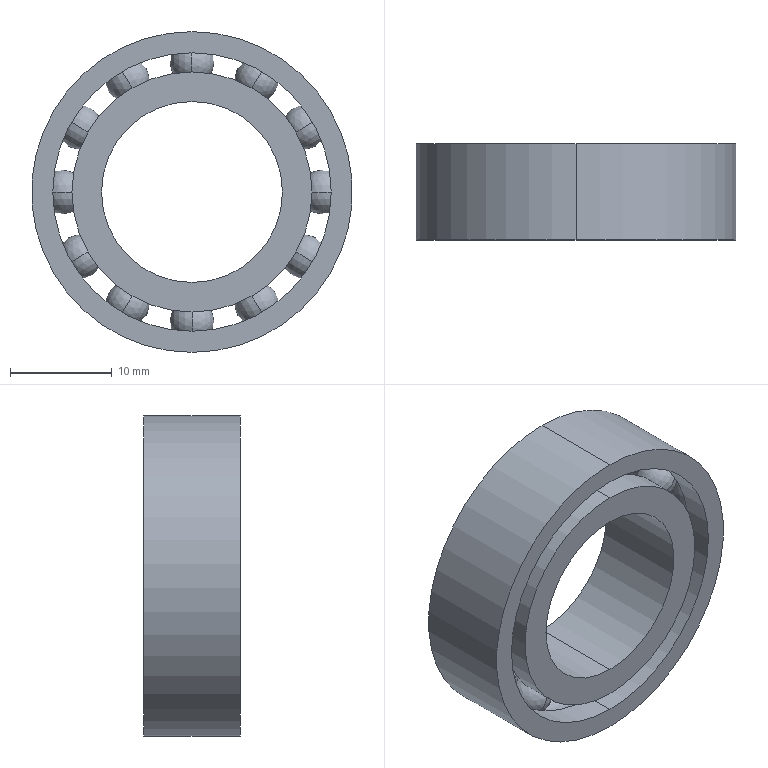Part | SolidWorks | features SavedExtBody 14 | 14 solids | 46 faces | box 31.502 x 9.43 x 31.502 mm | volume 3555 mm3 | sphere 24 | cylinder 12 | torus 6 | plane 4 | commonest cylinder face diameters 23.576 x4 27.342 x4 17.774 x2 31.502 x2
STEP:
#1=CARTESIAN_POINT('',(-11.024,-216.87,71.365));
#2=VERTEX_POINT('',#1);
#3=CARTESIAN_POINT('',(-11.024,-212.601,71.365));
#4=VERTEX_POINT('',#3);
#5=CARTESIAN_POINT('',(-11.024,-214.736,71.365));
#6=DIRECTION('',(0.5,0.,0.866));
#7=DIRECTION('',(0.866,0.,-0.5));
#8=AXIS2_PLACEMENT_3D('',#5,#6,#7);
#9=CIRCLE('',#8,2.135);
#10=EDGE_CURVE('',#2,#4,#9,.T.);
#11=ORIENTED_EDGE('',*,*,#10,.F.);
#12=CARTESIAN_POINT('',(-11.024,-214.736,71.365));
#13=DIRECTION('',(-0.5,0.,-0.866));
#14=DIRECTION('',(-0.866,0.,0.5));
#15=AXIS2_PLACEMENT_3D('',#12,#13,#14);
#16=CIRCLE('',#15,2.135);
#17=EDGE_CURVE('',#2,#4,#16,.T.);
#18=ORIENTED_EDGE('',*,*,#17,.T.);
#19=EDGE_LOOP('',(#11,#18));
#20=FACE_OUTER_BOUND('',#19,.T.);
#21=CARTESIAN_POINT('',(-11.024,-214.736,71.365));
#22=DIRECTION('',(-0.5,0.,-0.866));
#23=DIRECTION('',(0.866,0.,-0.5));
#24=AXIS2_PLACEMENT_3D('',#21,#22,#23);
#25=SPHERICAL_SURFACE('',#24,2.135);
#26=ADVANCED_FACE('',(#20),#25,.T.);
#27=ORIENTED_EDGE('',*,*,#17,.F.);
#28=ORIENTED_EDGE('',*,*,#10,.T.);
#29=EDGE_LOOP('',(#27,#28));
#30=FACE_OUTER_BOUND('',#29,.T.);
#31=CARTESIAN_POINT('',(-11.024,-214.736,71.365));
#32=DIRECTION('',(-0.5,0.,-0.866));
#33=DIRECTION('',(0.866,0.,-0.5));
#34=AXIS2_PLACEMENT_3D('',#31,#32,#33);
#35=SPHERICAL_SURFACE('',#34,2.135);
#36=ADVANCED_FACE('',(#30),#35,.T.);
#37=CLOSED_SHELL('',(#26,#36));
#38=MANIFOLD_SOLID_BREP('',#37);
#39=CARTESIAN_POINT('',(-6.365,-216.87,76.024));
#40=VERTEX_POINT('',#39);
#41=CARTESIAN_POINT('',(-6.365,-212.601,76.024));
#42=VERTEX_POINT('',#41);
#43=CARTESIAN_POINT('',(-6.365,-214.736,76.024));
#44=DIRECTION('',(0.866,0.,0.5));
#45=DIRECTION('',(0.5,0.,-0.866));
#46=AXIS2_PLACEMENT_3D('',#43,#44,#45);
#47=CIRCLE('',#46,2.135);
#48=EDGE_CURVE('',#40,#42,#47,.T.);
#49=ORIENTED_EDGE('',*,*,#48,.F.);
#50=CARTESIAN_POINT('',(-6.365,-214.736,76.024));
#51=DIRECTION('',(-0.866,0.,-0.5));
#52=DIRECTION('',(-0.5,0.,0.866));
#53=AXIS2_PLACEMENT_3D('',#50,#51,#52);
#54=CIRCLE('',#53,2.135);
#55=EDGE_CURVE('',#40,#42,#54,.T.);
#56=ORIENTED_EDGE('',*,*,#55,.T.);
#57=EDGE_LOOP('',(#49,#56));
#58=FACE_OUTER_BOUND('',#57,.T.);
#59=CARTESIAN_POINT('',(-6.365,-214.736,76.024));
#60=DIRECTION('',(-0.866,0.,-0.5));
#61=DIRECTION('',(0.5,0.,-0.866));
#62=AXIS2_PLACEMENT_3D('',#59,#60,#61);
#63=SPHERICAL_SURFACE('',#62,2.135);
#64=ADVANCED_FACE('',(#58),#63,.T.);
#65=ORIENTED_EDGE('',*,*,#55,.F.);
#66=ORIENTED_EDGE('',*,*,#48,.T.);
#67=EDGE_LOOP('',(#65,#66));
#68=FACE_OUTER_BOUND('',#67,.T.);
#69=CARTESIAN_POINT('',(-6.365,-214.736,76.024));
#70=DIRECTION('',(-0.866,0.,-0.5));
#71=DIRECTION('',(0.5,0.,-0.866));
#72=AXIS2_PLACEMENT_3D('',#69,#70,#71);
#73=SPHERICAL_SURFACE('',#72,2.135);
#74=ADVANCED_FACE('',(#68),#73,.T.);
#75=CLOSED_SHELL('',(#64,#74));
#76=MANIFOLD_SOLID_BREP('',#75);
#77=CARTESIAN_POINT('',(0.,-216.87,77.729));
#78=VERTEX_POINT('',#77);
#79=CARTESIAN_POINT('',(0.,-212.601,77.729));
#80=VERTEX_POINT('',#79);
#81=CARTESIAN_POINT('',(0.,-214.736,77.729));
#82=DIRECTION('',(1.,0.,0.));
#83=DIRECTION('',(0.,0.,-1.));
#84=AXIS2_PLACEMENT_3D('',#81,#82,#83);
#85=CIRCLE('',#84,2.135);
#86=EDGE_CURVE('',#78,#80,#85,.T.);
#87=ORIENTED_EDGE('',*,*,#86,.F.);
#88=CARTESIAN_POINT('',(0.,-214.736,77.729));
#89=DIRECTION('',(-1.,0.,0.));
#90=DIRECTION('',(0.,0.,1.));
#91=AXIS2_PLACEMENT_3D('',#88,#89,#90);
#92=CIRCLE('',#91,2.135);
#93=EDGE_CURVE('',#78,#80,#92,.T.);
#94=ORIENTED_EDGE('',*,*,#93,.T.);
#95=EDGE_LOOP('',(#87,#94));
#96=FACE_OUTER_BOUND('',#95,.T.);
#97=CARTESIAN_POINT('',(0.,-214.736,77.729));
#98=DIRECTION('',(-1.,0.,0.));
#99=DIRECTION('',(0.,0.,-1.));
#100=AXIS2_PLACEMENT_3D('',#97,#98,#99);
#101=SPHERICAL_SURFACE('',#100,2.135);
#102=ADVANCED_FACE('',(#96),#101,.T.);
#103=ORIENTED_EDGE('',*,*,#93,.F.);
#104=ORIENTED_EDGE('',*,*,#86,.T.);
#105=EDGE_LOOP('',(#103,#104));
#106=FACE_OUTER_BOUND('',#105,.T.);
#107=CARTESIAN_POINT('',(0.,-214.736,77.729));
#108=DIRECTION('',(-1.,0.,0.));
#109=DIRECTION('',(0.,0.,-1.));
#110=AXIS2_PLACEMENT_3D('',#107,#108,#109);
#111=SPHERICAL_SURFACE('',#110,2.135);
#112=ADVANCED_FACE('',(#106),#111,.T.);
#113=CLOSED_SHELL('',(#102,#112));
#114=MANIFOLD_SOLID_BREP('',#113);
#115=CARTESIAN_POINT('',(6.365,-216.87,76.024));
#116=VERTEX_POINT('',#115);
#117=CARTESIAN_POINT('',(6.365,-212.601,76.024));
#118=VERTEX_POINT('',#117);
#119=CARTESIAN_POINT('',(6.365,-214.736,76.024));
#120=DIRECTION('',(0.866,0.,-0.5));
#121=DIRECTION('',(-0.5,0.,-0.866));
#122=AXIS2_PLACEMENT_3D('',#119,#120,#121);
#123=CIRCLE('',#122,2.135);
#124=EDGE_CURVE('',#116,#118,#123,.T.);
#125=ORIENTED_EDGE('',*,*,#124,.F.);
#126=CARTESIAN_POINT('',(6.365,-214.736,76.024));
#127=DIRECTION('',(-0.866,0.,0.5));
#128=DIRECTION('',(0.5,0.,0.866));
#129=AXIS2_PLACEMENT_3D('',#126,#127,#128);
#130=CIRCLE('',#129,2.135);
#131=EDGE_CURVE('',#116,#118,#130,.T.);
#132=ORIENTED_EDGE('',*,*,#131,.T.);
#133=EDGE_LOOP('',(#125,#132));
#134=FACE_OUTER_BOUND('',#133,.T.);
#135=CARTESIAN_POINT('',(6.365,-214.736,76.024));
#136=DIRECTION('',(-0.866,0.,0.5));
#137=DIRECTION('',(-0.5,0.,-0.866));
#138=AXIS2_PLACEMENT_3D('',#135,#136,#137);
#139=SPHERICAL_SURFACE('',#138,2.135);
#140=ADVANCED_FACE('',(#134),#139,.T.);
#141=ORIENTED_EDGE('',*,*,#131,.F.);
#142=ORIENTED_EDGE('',*,*,#124,.T.);
#143=EDGE_LOOP('',(#141,#142));
#144=FACE_OUTER_BOUND('',#143,.T.);
#145=CARTESIAN_POINT('',(6.365,-214.736,76.024));
#146=DIRECTION('',(-0.866,0.,0.5));
#147=DIRECTION('',(-0.5,0.,-0.866));
#148=AXIS2_PLACEMENT_3D('',#145,#146,#147);
#149=SPHERICAL_SURFACE('',#148,2.135);
#150=ADVANCED_FACE('',(#144),#149,.T.);
#151=CLOSED_SHELL('',(#140,#150));
#152=MANIFOLD_SOLID_BREP('',#151);
#153=CARTESIAN_POINT('',(11.024,-216.87,71.365));
#154=VERTEX_POINT('',#153);
#155=CARTESIAN_POINT('',(11.024,-212.601,71.365));
#156=VERTEX_POINT('',#155);
#157=CARTESIAN_POINT('',(11.024,-214.736,71.365));
#158=DIRECTION('',(0.5,0.,-0.866));
#159=DIRECTION('',(-0.866,0.,-0.5));
#160=AXIS2_PLACEMENT_3D('',#157,#158,#159);
#161=CIRCLE('',#160,2.135);
#162=EDGE_CURVE('',#154,#156,#161,.T.);
#163=ORIENTED_EDGE('',*,*,#162,.F.);
#164=CARTESIAN_POINT('',(11.024,-214.736,71.365));
#165=DIRECTION('',(-0.5,0.,0.866));
#166=DIRECTION('',(0.866,0.,0.5));
#167=AXIS2_PLACEMENT_3D('',#164,#165,#166);
#168=CIRCLE('',#167,2.135);
#169=EDGE_CURVE('',#154,#156,#168,.T.);
#170=ORIENTED_EDGE('',*,*,#169,.T.);
#171=EDGE_LOOP('',(#163,#170));
#172=FACE_OUTER_BOUND('',#171,.T.);
#173=CARTESIAN_POINT('',(11.024,-214.736,71.365));
#174=DIRECTION('',(-0.5,0.,0.866));
#175=DIRECTION('',(-0.866,0.,-0.5));
#176=AXIS2_PLACEMENT_3D('',#173,#174,#175);
#177=SPHERICAL_SURFACE('',#176,2.135);
#178=ADVANCED_FACE('',(#172),#177,.T.);
#179=ORIENTED_EDGE('',*,*,#169,.F.);
#180=ORIENTED_EDGE('',*,*,#162,.T.);
#181=EDGE_LOOP('',(#179,#180));
#182=FACE_OUTER_BOUND('',#181,.T.);
#183=CARTESIAN_POINT('',(11.024,-214.736,71.365));
#184=DIRECTION('',(-0.5,0.,0.866));
#185=DIRECTION('',(-0.866,0.,-0.5));
#186=AXIS2_PLACEMENT_3D('',#183,#184,#185);
#187=SPHERICAL_SURFACE('',#186,2.135);
#188=ADVANCED_FACE('',(#182),#187,.T.);
#189=CLOSED_SHELL('',(#178,#188));
#190=MANIFOLD_SOLID_BREP('',#189);
#191=CARTESIAN_POINT('',(12.729,-216.87,65.));
#192=VERTEX_POINT('',#191);
#193=CARTESIAN_POINT('',(12.729,-212.601,65.));
#194=VERTEX_POINT('',#193);
#195=CARTESIAN_POINT('',(12.729,-214.736,65.));
#196=DIRECTION('',(0.,0.,-1.));
#197=DIRECTION('',(-1.,0.,0.));
#198=AXIS2_PLACEMENT_3D('',#195,#196,#197);
#199=CIRCLE('',#198,2.135);
#200=EDGE_CURVE('',#192,#194,#199,.T.);
#201=ORIENTED_EDGE('',*,*,#200,.F.);
#202=CARTESIAN_POINT('',(12.729,-214.736,65.));
#203=DIRECTION('',(0.,0.,1.));
#204=DIRECTION('',(1.,0.,0.));
#205=AXIS2_PLACEMENT_3D('',#202,#203,#204);
#206=CIRCLE('',#205,2.135);
#207=EDGE_CURVE('',#192,#194,#206,.T.);
#208=ORIENTED_EDGE('',*,*,#207,.T.);
#209=EDGE_LOOP('',(#201,#208));
#210=FACE_OUTER_BOUND('',#209,.T.);
#211=CARTESIAN_POINT('',(12.729,-214.736,65.));
#212=DIRECTION('',(0.,0.,1.));
#213=DIRECTION('',(-1.,0.,0.));
#214=AXIS2_PLACEMENT_3D('',#211,#212,#213);
#215=SPHERICAL_SURFACE('',#214,2.135);
#216=ADVANCED_FACE('',(#210),#215,.T.);
#217=ORIENTED_EDGE('',*,*,#207,.F.);
#218=ORIENTED_EDGE('',*,*,#200,.T.);
#219=EDGE_LOOP('',(#217,#218));
#220=FACE_OUTER_BOUND('',#219,.T.);
#221=CARTESIAN_POINT('',(12.729,-214.736,65.));
#222=DIRECTION('',(0.,0.,1.));
#223=DIRECTION('',(-1.,0.,0.));
#224=AXIS2_PLACEMENT_3D('',#221,#222,#223);
#225=SPHERICAL_SURFACE('',#224,2.135);
#226=ADVANCED_FACE('',(#220),#225,.T.);
#227=CLOSED_SHELL('',(#216,#226));
#228=MANIFOLD_SOLID_BREP('',#227);
#229=CARTESIAN_POINT('',(6.365,-216.87,53.976));
#230=VERTEX_POINT('',#229);
#231=CARTESIAN_POINT('',(6.365,-212.601,53.976));
#232=VERTEX_POINT('',#231);
#233=CARTESIAN_POINT('',(6.365,-214.736,53.976));
#234=DIRECTION('',(-0.866,0.,-0.5));
#235=DIRECTION('',(-0.5,0.,0.866));
#236=AXIS2_PLACEMENT_3D('',#233,#234,#235);
#237=CIRCLE('',#236,2.135);
#238=EDGE_CURVE('',#230,#232,#237,.T.);
#239=ORIENTED_EDGE('',*,*,#238,.F.);
#240=CARTESIAN_POINT('',(6.365,-214.736,53.976));
#241=DIRECTION('',(0.866,0.,0.5));
#242=DIRECTION('',(0.5,0.,-0.866));
#243=AXIS2_PLACEMENT_3D('',#240,#241,#242);
#244=CIRCLE('',#243,2.135);
#245=EDGE_CURVE('',#230,#232,#244,.T.);
#246=ORIENTED_EDGE('',*,*,#245,.T.);
#247=EDGE_LOOP('',(#239,#246));
#248=FACE_OUTER_BOUND('',#247,.T.);
#249=CARTESIAN_POINT('',(6.365,-214.736,53.976));
#250=DIRECTION('',(0.866,0.,0.5));
#251=DIRECTION('',(-0.5,0.,0.866));
#252=AXIS2_PLACEMENT_3D('',#249,#250,#251);
#253=SPHERICAL_SURFACE('',#252,2.135);
#254=ADVANCED_FACE('',(#248),#253,.T.);
#255=ORIENTED_EDGE('',*,*,#245,.F.);
#256=ORIENTED_EDGE('',*,*,#238,.T.);
#257=EDGE_LOOP('',(#255,#256));
#258=FACE_OUTER_BOUND('',#257,.T.);
#259=CARTESIAN_POINT('',(6.365,-214.736,53.976));
#260=DIRECTION('',(0.866,0.,0.5));
#261=DIRECTION('',(-0.5,0.,0.866));
#262=AXIS2_PLACEMENT_3D('',#259,#260,#261);
#263=SPHERICAL_SURFACE('',#262,2.135);
#264=ADVANCED_FACE('',(#258),#263,.T.);
#265=CLOSED_SHELL('',(#254,#264));
#266=MANIFOLD_SOLID_BREP('',#265);
#267=CARTESIAN_POINT('',(0.,-216.87,52.271));
#268=VERTEX_POINT('',#267);
#269=CARTESIAN_POINT('',(0.,-212.601,52.271));
#270=VERTEX_POINT('',#269);
#271=CARTESIAN_POINT('',(0.,-214.736,52.271));
#272=DIRECTION('',(-1.,0.,0.));
#273=DIRECTION('',(0.,0.,1.));
#274=AXIS2_PLACEMENT_3D('',#271,#272,#273);
#275=CIRCLE('',#274,2.135);
#276=EDGE_CURVE('',#268,#270,#275,.T.);
#277=ORIENTED_EDGE('',*,*,#276,.F.);
#278=CARTESIAN_POINT('',(0.,-214.736,52.271));
#279=DIRECTION('',(1.,0.,0.));
#280=DIRECTION('',(0.,0.,-1.));
#281=AXIS2_PLACEMENT_3D('',#278,#279,#280);
#282=CIRCLE('',#281,2.135);
#283=EDGE_CURVE('',#268,#270,#282,.T.);
#284=ORIENTED_EDGE('',*,*,#283,.T.);
#285=EDGE_LOOP('',(#277,#284));
#286=FACE_OUTER_BOUND('',#285,.T.);
#287=CARTESIAN_POINT('',(0.,-214.736,52.271));
#288=DIRECTION('',(1.,0.,0.));
#289=DIRECTION('',(0.,0.,1.));
#290=AXIS2_PLACEMENT_3D('',#287,#288,#289);
#291=SPHERICAL_SURFACE('',#290,2.135);
#292=ADVANCED_FACE('',(#286),#291,.T.);
#293=ORIENTED_EDGE('',*,*,#283,.F.);
#294=ORIENTED_EDGE('',*,*,#276,.T.);
#295=EDGE_LOOP('',(#293,#294));
#296=FACE_OUTER_BOUND('',#295,.T.);
#297=CARTESIAN_POINT('',(0.,-214.736,52.271));
#298=DIRECTION('',(1.,0.,0.));
#299=DIRECTION('',(0.,0.,1.));
#300=AXIS2_PLACEMENT_3D('',#297,#298,#299);
#301=SPHERICAL_SURFACE('',#300,2.135);
#302=ADVANCED_FACE('',(#296),#301,.T.);
#303=CLOSED_SHELL('',(#292,#302));
#304=MANIFOLD_SOLID_BREP('',#303);
#305=CARTESIAN_POINT('',(-6.365,-216.87,53.976));
#306=VERTEX_POINT('',#305);
#307=CARTESIAN_POINT('',(-6.365,-212.601,53.976));
#308=VERTEX_POINT('',#307);
#309=CARTESIAN_POINT('',(-6.365,-214.736,53.976));
#310=DIRECTION('',(-0.866,0.,0.5));
#311=DIRECTION('',(0.5,0.,0.866));
#312=AXIS2_PLACEMENT_3D('',#309,#310,#311);
#313=CIRCLE('',#312,2.135);
#314=EDGE_CURVE('',#306,#308,#313,.T.);
#315=ORIENTED_EDGE('',*,*,#314,.F.);
#316=CARTESIAN_POINT('',(-6.365,-214.736,53.976));
#317=DIRECTION('',(0.866,0.,-0.5));
#318=DIRECTION('',(-0.5,0.,-0.866));
#319=AXIS2_PLACEMENT_3D('',#316,#317,#318);
#320=CIRCLE('',#319,2.135);
#321=EDGE_CURVE('',#306,#308,#320,.T.);
#322=ORIENTED_EDGE('',*,*,#321,.T.);
#323=EDGE_LOOP('',(#315,#322));
#324=FACE_OUTER_BOUND('',#323,.T.);
#325=CARTESIAN_POINT('',(-6.365,-214.736,53.976));
#326=DIRECTION('',(0.866,0.,-0.5));
#327=DIRECTION('',(0.5,0.,0.866));
#328=AXIS2_PLACEMENT_3D('',#325,#326,#327);
#329=SPHERICAL_SURFACE('',#328,2.135);
#330=ADVANCED_FACE('',(#324),#329,.T.);
#331=ORIENTED_EDGE('',*,*,#321,.F.);
#332=ORIENTED_EDGE('',*,*,#314,.T.);
#333=EDGE_LOOP('',(#331,#332));
#334=FACE_OUTER_BOUND('',#333,.T.);
#335=CARTESIAN_POINT('',(-6.365,-214.736,53.976));
#336=DIRECTION('',(0.866,0.,-0.5));
#337=DIRECTION('',(0.5,0.,0.866));
#338=AXIS2_PLACEMENT_3D('',#335,#336,#337);
#339=SPHERICAL_SURFACE('',#338,2.135);
#340=ADVANCED_FACE('',(#334),#339,.T.);
#341=CLOSED_SHELL('',(#330,#340));
#342=MANIFOLD_SOLID_BREP('',#341);
#343=CARTESIAN_POINT('',(-11.024,-216.87,58.635));
#344=VERTEX_POINT('',#343);
#345=CARTESIAN_POINT('',(-11.024,-212.601,58.635));
#346=VERTEX_POINT('',#345);
#347=CARTESIAN_POINT('',(-11.024,-214.736,58.635));
#348=DIRECTION('',(-0.5,0.,0.866));
#349=DIRECTION('',(0.866,0.,0.5));
#350=AXIS2_PLACEMENT_3D('',#347,#348,#349);
#351=CIRCLE('',#350,2.135);
#352=EDGE_CURVE('',#344,#346,#351,.T.);
#353=ORIENTED_EDGE('',*,*,#352,.F.);
#354=CARTESIAN_POINT('',(-11.024,-214.736,58.635));
#355=DIRECTION('',(0.5,0.,-0.866));
#356=DIRECTION('',(-0.866,0.,-0.5));
#357=AXIS2_PLACEMENT_3D('',#354,#355,#356);
#358=CIRCLE('',#357,2.135);
#359=EDGE_CURVE('',#344,#346,#358,.T.);
#360=ORIENTED_EDGE('',*,*,#359,.T.);
#361=EDGE_LOOP('',(#353,#360));
#362=FACE_OUTER_BOUND('',#361,.T.);
#363=CARTESIAN_POINT('',(-11.024,-214.736,58.635));
#364=DIRECTION('',(0.5,0.,-0.866));
#365=DIRECTION('',(0.866,0.,0.5));
#366=AXIS2_PLACEMENT_3D('',#363,#364,#365);
#367=SPHERICAL_SURFACE('',#366,2.135);
#368=ADVANCED_FACE('',(#362),#367,.T.);
#369=ORIENTED_EDGE('',*,*,#359,.F.);
#370=ORIENTED_EDGE('',*,*,#352,.T.);
#371=EDGE_LOOP('',(#369,#370));
#372=FACE_OUTER_BOUND('',#371,.T.);
#373=CARTESIAN_POINT('',(-11.024,-214.736,58.635));
#374=DIRECTION('',(0.5,0.,-0.866));
#375=DIRECTION('',(0.866,0.,0.5));
#376=AXIS2_PLACEMENT_3D('',#373,#374,#375);
#377=SPHERICAL_SURFACE('',#376,2.135);
#378=ADVANCED_FACE('',(#372),#377,.T.);
#379=CLOSED_SHELL('',(#368,#378));
#380=MANIFOLD_SOLID_BREP('',#379);
#381=CARTESIAN_POINT('',(-12.729,-216.87,65.));
#382=VERTEX_POINT('',#381);
#383=CARTESIAN_POINT('',(-12.729,-212.601,65.));
#384=VERTEX_POINT('',#383);
#385=CARTESIAN_POINT('',(-12.729,-214.736,65.));
#386=DIRECTION('',(0.,0.,1.));
#387=DIRECTION('',(1.,0.,0.));
#388=AXIS2_PLACEMENT_3D('',#385,#386,#387);
#389=CIRCLE('',#388,2.135);
#390=EDGE_CURVE('',#382,#384,#389,.T.);
#391=ORIENTED_EDGE('',*,*,#390,.F.);
#392=CARTESIAN_POINT('',(-12.729,-214.736,65.));
#393=DIRECTION('',(0.,0.,-1.));
#394=DIRECTION('',(-1.,0.,0.));
#395=AXIS2_PLACEMENT_3D('',#392,#393,#394);
#396=CIRCLE('',#395,2.135);
#397=EDGE_CURVE('',#382,#384,#396,.T.);
#398=ORIENTED_EDGE('',*,*,#397,.T.);
#399=EDGE_LOOP('',(#391,#398));
#400=FACE_OUTER_BOUND('',#399,.T.);
#401=CARTESIAN_POINT('',(-12.729,-214.736,65.));
#402=DIRECTION('',(0.,0.,-1.));
#403=DIRECTION('',(1.,0.,0.));
#404=AXIS2_PLACEMENT_3D('',#401,#402,#403);
#405=SPHERICAL_SURFACE('',#404,2.135);
#406=ADVANCED_FACE('',(#400),#405,.T.);
#407=ORIENTED_EDGE('',*,*,#397,.F.);
#408=ORIENTED_EDGE('',*,*,#390,.T.);
#409=EDGE_LOOP('',(#407,#408));
#410=FACE_OUTER_BOUND('',#409,.T.);
#411=CARTESIAN_POINT('',(-12.729,-214.736,65.));
#412=DIRECTION('',(0.,0.,-1.));
#413=DIRECTION('',(1.,0.,0.));
#414=AXIS2_PLACEMENT_3D('',#411,#412,#413);
#415=SPHERICAL_SURFACE('',#414,2.135);
#416=ADVANCED_FACE('',(#410),#415,.T.);
#417=CLOSED_SHELL('',(#406,#416));
#418=MANIFOLD_SOLID_BREP('',#417);
#419=CARTESIAN_POINT('',(0.,-216.652,53.212));
#420=VERTEX_POINT('',#419);
#421=CARTESIAN_POINT('',(0.,-214.736,54.405));
#422=VERTEX_POINT('',#421);
#423=CARTESIAN_POINT('',(0.,-214.736,52.271));
#424=DIRECTION('',(-1.,0.,0.));
#425=DIRECTION('',(0.,0.,1.));
#426=AXIS2_PLACEMENT_3D('',#423,#424,#425);
#427=CIRCLE('',#426,2.135);
#428=EDGE_CURVE('',#420,#422,#427,.T.);
#429=ORIENTED_EDGE('',*,*,#428,.T.);
#430=CARTESIAN_POINT('',(0.,-214.736,75.595));
#431=VERTEX_POINT('',#430);
#432=CARTESIAN_POINT('',(0.,-214.736,65.));
#433=DIRECTION('',(0.,-1.,0.));
#434=DIRECTION('',(0.,0.,-1.));
#435=AXIS2_PLACEMENT_3D('',#432,#433,#434);
#436=CIRCLE('',#435,10.595);
#437=EDGE_CURVE('',#422,#431,#436,.T.);
#438=ORIENTED_EDGE('',*,*,#437,.T.);
#439=CARTESIAN_POINT('',(0.,-216.652,76.788));
#440=VERTEX_POINT('',#439);
#441=CARTESIAN_POINT('',(0.,-214.736,77.729));
#442=DIRECTION('',(1.,0.,0.));
#443=DIRECTION('',(0.,0.,-1.));
#444=AXIS2_PLACEMENT_3D('',#441,#442,#443);
#445=CIRCLE('',#444,2.135);
#446=EDGE_CURVE('',#440,#431,#445,.T.);
#447=ORIENTED_EDGE('',*,*,#446,.F.);
#448=CARTESIAN_POINT('',(0.,-216.652,65.));
#449=DIRECTION('',(0.,-1.,0.));
#450=DIRECTION('',(0.,0.,-1.));
#451=AXIS2_PLACEMENT_3D('',#448,#449,#450);
#452=CIRCLE('',#451,11.788);
#453=EDGE_CURVE('',#420,#440,#452,.T.);
#454=ORIENTED_EDGE('',*,*,#453,.F.);
#455=EDGE_LOOP('',(#429,#438,#447,#454));
#456=FACE_OUTER_BOUND('',#455,.T.);
#457=CARTESIAN_POINT('',(0.,-214.736,65.));
#458=DIRECTION('',(0.,-1.,0.));
#459=DIRECTION('',(0.,0.,-1.));
#460=AXIS2_PLACEMENT_3D('',#457,#458,#459);
#461=TOROIDAL_SURFACE('',#460,12.729,2.135);
#462=ADVANCED_FACE('',(#456),#461,.F.);
#463=ORIENTED_EDGE('',*,*,#446,.T.);
#464=CARTESIAN_POINT('',(0.,-214.736,65.));
#465=DIRECTION('',(0.,-1.,0.));
#466=DIRECTION('',(0.,0.,-1.));
#467=AXIS2_PLACEMENT_3D('',#464,#465,#466);
#468=CIRCLE('',#467,10.595);
#469=EDGE_CURVE('',#431,#422,#468,.T.);
#470=ORIENTED_EDGE('',*,*,#469,.T.);
#471=ORIENTED_EDGE('',*,*,#428,.F.);
#472=CARTESIAN_POINT('',(0.,-216.652,65.));
#473=DIRECTION('',(0.,-1.,0.));
#474=DIRECTION('',(0.,0.,-1.));
#475=AXIS2_PLACEMENT_3D('',#472,#473,#474);
#476=CIRCLE('',#475,11.788);
#477=EDGE_CURVE('',#440,#420,#476,.T.);
#478=ORIENTED_EDGE('',*,*,#477,.F.);
#479=EDGE_LOOP('',(#463,#470,#471,#478));
#480=FACE_OUTER_BOUND('',#479,.T.);
#481=CARTESIAN_POINT('',(0.,-214.736,65.));
#482=DIRECTION('',(0.,-1.,0.));
#483=DIRECTION('',(0.,0.,-1.));
#484=AXIS2_PLACEMENT_3D('',#481,#482,#483);
#485=TOROIDAL_SURFACE('',#484,12.729,2.135);
#486=ADVANCED_FACE('',(#480),#485,.F.);
#487=CARTESIAN_POINT('',(0.,-210.021,73.887));
#488=VERTEX_POINT('',#487);
#489=CARTESIAN_POINT('',(0.,-210.021,56.113));
#490=VERTEX_POINT('',#489);
#491=CARTESIAN_POINT('',(0.,-210.021,65.));
#492=DIRECTION('',(0.,-1.,0.));
#493=DIRECTION('',(0.,0.,-1.));
#494=AXIS2_PLACEMENT_3D('',#491,#492,#493);
#495=CIRCLE('',#494,8.887);
#496=EDGE_CURVE('',#488,#490,#495,.T.);
#497=ORIENTED_EDGE('',*,*,#496,.F.);
#498=CARTESIAN_POINT('',(0.,-219.451,73.887));
#499=VERTEX_POINT('',#498);
#500=CARTESIAN_POINT('',(0.,-253.035,73.887));
#501=DIRECTION('',(0.,-1.,0.));
#502=VECTOR('',#501,1000.);
#503=LINE('',#500,#502);
#504=EDGE_CURVE('',#488,#499,#503,.T.);
#505=ORIENTED_EDGE('',*,*,#504,.T.);
#506=CARTESIAN_POINT('',(0.,-219.451,56.113));
#507=VERTEX_POINT('',#506);
#508=CARTESIAN_POINT('',(0.,-219.451,65.));
#509=DIRECTION('',(0.,-1.,0.));
#510=DIRECTION('',(0.,0.,-1.));
#511=AXIS2_PLACEMENT_3D('',#508,#509,#510);
#512=CIRCLE('',#511,8.887);
#513=EDGE_CURVE('',#499,#507,#512,.T.);
#514=ORIENTED_EDGE('',*,*,#513,.T.);
#515=CARTESIAN_POINT('',(0.,-253.035,56.113));
#516=DIRECTION('',(0.,-1.,0.));
#517=VECTOR('',#516,1000.);
#518=LINE('',#515,#517);
#519=EDGE_CURVE('',#490,#507,#518,.T.);
#520=ORIENTED_EDGE('',*,*,#519,.F.);
#521=EDGE_LOOP('',(#497,#505,#514,#520));
#522=FACE_OUTER_BOUND('',#521,.T.);
#523=CARTESIAN_POINT('',(0.,-253.035,65.));
#524=DIRECTION('',(0.,-1.,0.));
#525=DIRECTION('',(0.,0.,-1.));
#526=AXIS2_PLACEMENT_3D('',#523,#524,#525);
#527=CYLINDRICAL_SURFACE('',#526,8.887);
#528=ADVANCED_FACE('',(#522),#527,.F.);
#529=ORIENTED_EDGE('',*,*,#453,.T.);
#530=CARTESIAN_POINT('',(0.,-219.451,76.788));
#531=VERTEX_POINT('',#530);
#532=CARTESIAN_POINT('',(0.,-253.035,76.788));
#533=DIRECTION('',(0.,-1.,0.));
#534=VECTOR('',#533,1000.);
#535=LINE('',#532,#534);
#536=EDGE_CURVE('',#440,#531,#535,.T.);
#537=ORIENTED_EDGE('',*,*,#536,.T.);
#538=CARTESIAN_POINT('',(0.,-219.451,53.212));
#539=VERTEX_POINT('',#538);
#540=CARTESIAN_POINT('',(0.,-219.451,65.));
#541=DIRECTION('',(0.,-1.,0.));
#542=DIRECTION('',(0.,0.,-1.));
#543=AXIS2_PLACEMENT_3D('',#540,#541,#542);
#544=CIRCLE('',#543,11.788);
#545=EDGE_CURVE('',#539,#531,#544,.T.);
#546=ORIENTED_EDGE('',*,*,#545,.F.);
#547=CARTESIAN_POINT('',(0.,-253.035,53.212));
#548=DIRECTION('',(0.,-1.,0.));
#549=VECTOR('',#548,1000.);
#550=LINE('',#547,#549);
#551=EDGE_CURVE('',#420,#539,#550,.T.);
#552=ORIENTED_EDGE('',*,*,#551,.F.);
#553=EDGE_LOOP('',(#529,#537,#546,#552));
#554=FACE_OUTER_BOUND('',#553,.T.);
#555=CARTESIAN_POINT('',(0.,-253.035,65.));
#556=DIRECTION('',(0.,-1.,0.));
#557=DIRECTION('',(0.,0.,-1.));
#558=AXIS2_PLACEMENT_3D('',#555,#556,#557);
#559=CYLINDRICAL_SURFACE('',#558,11.788);
#560=ADVANCED_FACE('',(#554),#559,.T.);
#561=ORIENTED_EDGE('',*,*,#469,.F.);
#562=CARTESIAN_POINT('',(0.,-212.82,76.788));
#563=VERTEX_POINT('',#562);
#564=CARTESIAN_POINT('',(0.,-214.736,77.729));
#565=DIRECTION('',(1.,0.,0.));
#566=DIRECTION('',(0.,0.,-1.));
#567=AXIS2_PLACEMENT_3D('',#564,#565,#566);
#568=CIRCLE('',#567,2.135);
#569=EDGE_CURVE('',#431,#563,#568,.T.);
#570=ORIENTED_EDGE('',*,*,#569,.T.);
#571=CARTESIAN_POINT('',(0.,-212.82,53.212));
#572=VERTEX_POINT('',#571);
#573=CARTESIAN_POINT('',(0.,-212.82,65.));
#574=DIRECTION('',(0.,-1.,0.));
#575=DIRECTION('',(0.,0.,-1.));
#576=AXIS2_PLACEMENT_3D('',#573,#574,#575);
#577=CIRCLE('',#576,11.788);
#578=EDGE_CURVE('',#563,#572,#577,.T.);
#579=ORIENTED_EDGE('',*,*,#578,.T.);
#580=CARTESIAN_POINT('',(0.,-214.736,52.271));
#581=DIRECTION('',(-1.,0.,0.));
#582=DIRECTION('',(0.,0.,1.));
#583=AXIS2_PLACEMENT_3D('',#580,#581,#582);
#584=CIRCLE('',#583,2.135);
#585=EDGE_CURVE('',#422,#572,#584,.T.);
#586=ORIENTED_EDGE('',*,*,#585,.F.);
#587=EDGE_LOOP('',(#561,#570,#579,#586));
#588=FACE_OUTER_BOUND('',#587,.T.);
#589=CARTESIAN_POINT('',(0.,-214.736,65.));
#590=DIRECTION('',(0.,-1.,0.));
#591=DIRECTION('',(0.,0.,-1.));
#592=AXIS2_PLACEMENT_3D('',#589,#590,#591);
#593=TOROIDAL_SURFACE('',#592,12.729,2.135);
#594=ADVANCED_FACE('',(#588),#593,.F.);
#595=CARTESIAN_POINT('',(0.,-210.021,53.212));
#596=VERTEX_POINT('',#595);
#597=CARTESIAN_POINT('',(0.,-210.021,76.788));
#598=VERTEX_POINT('',#597);
#599=CARTESIAN_POINT('',(0.,-210.021,65.));
#600=DIRECTION('',(0.,-1.,0.));
#601=DIRECTION('',(0.,0.,-1.));
#602=AXIS2_PLACEMENT_3D('',#599,#600,#601);
#603=CIRCLE('',#602,11.788);
#604=EDGE_CURVE('',#596,#598,#603,.T.);
#605=ORIENTED_EDGE('',*,*,#604,.T.);
#606=CARTESIAN_POINT('',(0.,-253.035,76.788));
#607=DIRECTION('',(0.,-1.,0.));
#608=VECTOR('',#607,1000.);
#609=LINE('',#606,#608);
#610=EDGE_CURVE('',#598,#563,#609,.T.);
#611=ORIENTED_EDGE('',*,*,#610,.T.);
#612=CARTESIAN_POINT('',(0.,-212.82,65.));
#613=DIRECTION('',(0.,-1.,0.));
#614=DIRECTION('',(0.,0.,-1.));
#615=AXIS2_PLACEMENT_3D('',#612,#613,#614);
#616=CIRCLE('',#615,11.788);
#617=EDGE_CURVE('',#572,#563,#616,.T.);
#618=ORIENTED_EDGE('',*,*,#617,.F.);
#619=CARTESIAN_POINT('',(0.,-253.035,53.212));
#620=DIRECTION('',(0.,-1.,0.));
#621=VECTOR('',#620,1000.);
#622=LINE('',#619,#621);
#623=EDGE_CURVE('',#596,#572,#622,.T.);
#624=ORIENTED_EDGE('',*,*,#623,.F.);
#625=EDGE_LOOP('',(#605,#611,#618,#624));
#626=FACE_OUTER_BOUND('',#625,.T.);
#627=CARTESIAN_POINT('',(0.,-253.035,65.));
#628=DIRECTION('',(0.,-1.,0.));
#629=DIRECTION('',(0.,0.,-1.));
#630=AXIS2_PLACEMENT_3D('',#627,#628,#629);
#631=CYLINDRICAL_SURFACE('',#630,11.788);
#632=ADVANCED_FACE('',(#626),#631,.T.);
#633=ORIENTED_EDGE('',*,*,#604,.F.);
#634=CARTESIAN_POINT('',(0.,-210.021,65.));
#635=DIRECTION('',(0.,-1.,0.));
#636=DIRECTION('',(0.,0.,-1.));
#637=AXIS2_PLACEMENT_3D('',#634,#635,#636);
#638=CIRCLE('',#637,11.788);
#639=EDGE_CURVE('',#598,#596,#638,.T.);
#640=ORIENTED_EDGE('',*,*,#639,.F.);
#641=EDGE_LOOP('',(#633,#640));
#642=FACE_OUTER_BOUND('',#641,.T.);
#643=CARTESIAN_POINT('',(0.,-210.021,65.));
#644=DIRECTION('',(0.,-1.,0.));
#645=DIRECTION('',(0.,0.,-1.));
#646=AXIS2_PLACEMENT_3D('',#643,#644,#645);
#647=CIRCLE('',#646,8.887);
#648=EDGE_CURVE('',#490,#488,#647,.T.);
#649=ORIENTED_EDGE('',*,*,#648,.T.);
#650=ORIENTED_EDGE('',*,*,#496,.T.);
#651=EDGE_LOOP('',(#649,#650));
#652=FACE_BOUND('',#651,.T.);
#653=CARTESIAN_POINT('',(-11.788,-210.021,65.));
#654=DIRECTION('',(0.,-1.,0.));
#655=DIRECTION('',(0.,0.,-1.));
#656=AXIS2_PLACEMENT_3D('',#653,#654,#655);
#657=PLANE('',#656);
#658=ADVANCED_FACE('',(#642,#652),#657,.F.);
#659=ORIENTED_EDGE('',*,*,#610,.F.);
#660=ORIENTED_EDGE('',*,*,#639,.T.);
#661=ORIENTED_EDGE('',*,*,#623,.T.);
#662=ORIENTED_EDGE('',*,*,#578,.F.);
#663=EDGE_LOOP('',(#659,#660,#661,#662));
#664=FACE_OUTER_BOUND('',#663,.T.);
#665=CARTESIAN_POINT('',(0.,-253.035,65.));
#666=DIRECTION('',(0.,-1.,0.));
#667=DIRECTION('',(0.,0.,-1.));
#668=AXIS2_PLACEMENT_3D('',#665,#666,#667);
#669=CYLINDRICAL_SURFACE('',#668,11.788);
#670=ADVANCED_FACE('',(#664),#669,.T.);
#671=ORIENTED_EDGE('',*,*,#437,.F.);
#672=ORIENTED_EDGE('',*,*,#585,.T.);
#673=ORIENTED_EDGE('',*,*,#617,.T.);
#674=ORIENTED_EDGE('',*,*,#569,.F.);
#675=EDGE_LOOP('',(#671,#672,#673,#674));
#676=FACE_OUTER_BOUND('',#675,.T.);
#677=CARTESIAN_POINT('',(0.,-214.736,65.));
#678=DIRECTION('',(0.,-1.,0.));
#679=DIRECTION('',(0.,0.,-1.));
#680=AXIS2_PLACEMENT_3D('',#677,#678,#679);
#681=TOROIDAL_SURFACE('',#680,12.729,2.135);
#682=ADVANCED_FACE('',(#676),#681,.F.);
#683=ORIENTED_EDGE('',*,*,#536,.F.);
#684=ORIENTED_EDGE('',*,*,#477,.T.);
#685=ORIENTED_EDGE('',*,*,#551,.T.);
#686=CARTESIAN_POINT('',(0.,-219.451,65.));
#687=DIRECTION('',(0.,-1.,0.));
#688=DIRECTION('',(0.,0.,-1.));
#689=AXIS2_PLACEMENT_3D('',#686,#687,#688);
#690=CIRCLE('',#689,11.788);
#691=EDGE_CURVE('',#531,#539,#690,.T.);
#692=ORIENTED_EDGE('',*,*,#691,.F.);
#693=EDGE_LOOP('',(#683,#684,#685,#692));
#694=FACE_OUTER_BOUND('',#693,.T.);
#695=CARTESIAN_POINT('',(0.,-253.035,65.));
#696=DIRECTION('',(0.,-1.,0.));
#697=DIRECTION('',(0.,0.,-1.));
#698=AXIS2_PLACEMENT_3D('',#695,#696,#697);
#699=CYLINDRICAL_SURFACE('',#698,11.788);
#700=ADVANCED_FACE('',(#694),#699,.T.);
#701=CARTESIAN_POINT('',(0.,-219.451,65.));
#702=DIRECTION('',(0.,-1.,0.));
#703=DIRECTION('',(0.,0.,-1.));
#704=AXIS2_PLACEMENT_3D('',#701,#702,#703);
#705=CIRCLE('',#704,8.887);
#706=EDGE_CURVE('',#507,#499,#705,.T.);
#707=ORIENTED_EDGE('',*,*,#706,.F.);
#708=ORIENTED_EDGE('',*,*,#513,.F.);
#709=EDGE_LOOP('',(#707,#708));
#710=FACE_BOUND('',#709,.T.);
#711=ORIENTED_EDGE('',*,*,#545,.T.);
#712=ORIENTED_EDGE('',*,*,#691,.T.);
#713=EDGE_LOOP('',(#711,#712));
#714=FACE_OUTER_BOUND('',#713,.T.);
#715=CARTESIAN_POINT('',(-11.788,-219.451,65.));
#716=DIRECTION('',(0.,1.,0.));
#717=DIRECTION('',(0.,0.,1.));
#718=AXIS2_PLACEMENT_3D('',#715,#716,#717);
#719=PLANE('',#718);
#720=ADVANCED_FACE('',(#710,#714),#719,.F.);
#721=ORIENTED_EDGE('',*,*,#504,.F.);
#722=ORIENTED_EDGE('',*,*,#648,.F.);
#723=ORIENTED_EDGE('',*,*,#519,.T.);
#724=ORIENTED_EDGE('',*,*,#706,.T.);
#725=EDGE_LOOP('',(#721,#722,#723,#724));
#726=FACE_OUTER_BOUND('',#725,.T.);
#727=CARTESIAN_POINT('',(0.,-253.035,65.));
#728=DIRECTION('',(0.,-1.,0.));
#729=DIRECTION('',(0.,0.,-1.));
#730=AXIS2_PLACEMENT_3D('',#727,#728,#729);
#731=CYLINDRICAL_SURFACE('',#730,8.887);
#732=ADVANCED_FACE('',(#726),#731,.F.);
#733=CLOSED_SHELL('',(#462,#486,#528,#560,#594,#632,#658,#670,#682,#700,#720,#732));
#734=MANIFOLD_SOLID_BREP('',#733);
#735=CARTESIAN_POINT('',(0.,-210.021,78.671));
#736=VERTEX_POINT('',#735);
#737=CARTESIAN_POINT('',(0.,-210.021,51.329));
#738=VERTEX_POINT('',#737);
#739=CARTESIAN_POINT('',(0.,-210.021,65.));
#740=DIRECTION('',(0.,-1.,0.));
#741=DIRECTION('',(0.,0.,-1.));
#742=AXIS2_PLACEMENT_3D('',#739,#740,#741);
#743=CIRCLE('',#742,13.671);
#744=EDGE_CURVE('',#736,#738,#743,.T.);
#745=ORIENTED_EDGE('',*,*,#744,.F.);
#746=CARTESIAN_POINT('',(0.,-212.82,78.671));
#747=VERTEX_POINT('',#746);
#748=CARTESIAN_POINT('',(0.,-253.035,78.671));
#749=DIRECTION('',(0.,-1.,0.));
#750=VECTOR('',#749,1000.);
#751=LINE('',#748,#750);
#752=EDGE_CURVE('',#736,#747,#751,.T.);
#753=ORIENTED_EDGE('',*,*,#752,.T.);
#754=CARTESIAN_POINT('',(0.,-212.82,51.329));
#755=VERTEX_POINT('',#754);
#756=CARTESIAN_POINT('',(0.,-212.82,65.));
#757=DIRECTION('',(0.,-1.,0.));
#758=DIRECTION('',(0.,0.,-1.));
#759=AXIS2_PLACEMENT_3D('',#756,#757,#758);
#760=CIRCLE('',#759,13.671);
#761=EDGE_CURVE('',#747,#755,#760,.T.);
#762=ORIENTED_EDGE('',*,*,#761,.T.);
#763=CARTESIAN_POINT('',(0.,-253.035,51.329));
#764=DIRECTION('',(0.,-1.,0.));
#765=VECTOR('',#764,1000.);
#766=LINE('',#763,#765);
#767=EDGE_CURVE('',#738,#755,#766,.T.);
#768=ORIENTED_EDGE('',*,*,#767,.F.);
#769=EDGE_LOOP('',(#745,#753,#762,#768));
#770=FACE_OUTER_BOUND('',#769,.T.);
#771=CARTESIAN_POINT('',(0.,-253.035,65.));
#772=DIRECTION('',(0.,-1.,0.));
#773=DIRECTION('',(0.,0.,-1.));
#774=AXIS2_PLACEMENT_3D('',#771,#772,#773);
#775=CYLINDRICAL_SURFACE('',#774,13.671);
#776=ADVANCED_FACE('',(#770),#775,.F.);
#777=ORIENTED_EDGE('',*,*,#761,.F.);
#778=CARTESIAN_POINT('',(0.,-216.652,78.671));
#779=VERTEX_POINT('',#778);
#780=CARTESIAN_POINT('',(0.,-214.736,77.729));
#781=DIRECTION('',(1.,0.,0.));
#782=DIRECTION('',(0.,0.,-1.));
#783=AXIS2_PLACEMENT_3D('',#780,#781,#782);
#784=CIRCLE('',#783,2.135);
#785=EDGE_CURVE('',#747,#779,#784,.T.);
#786=ORIENTED_EDGE('',*,*,#785,.T.);
#787=CARTESIAN_POINT('',(0.,-216.652,51.329));
#788=VERTEX_POINT('',#787);
#789=CARTESIAN_POINT('',(0.,-216.652,65.));
#790=DIRECTION('',(0.,-1.,0.));
#791=DIRECTION('',(0.,0.,-1.));
#792=AXIS2_PLACEMENT_3D('',#789,#790,#791);
#793=CIRCLE('',#792,13.671);
#794=EDGE_CURVE('',#779,#788,#793,.T.);
#795=ORIENTED_EDGE('',*,*,#794,.T.);
#796=CARTESIAN_POINT('',(0.,-214.736,52.271));
#797=DIRECTION('',(-1.,0.,0.));
#798=DIRECTION('',(0.,0.,1.));
#799=AXIS2_PLACEMENT_3D('',#796,#797,#798);
#800=CIRCLE('',#799,2.135);
#801=EDGE_CURVE('',#755,#788,#800,.T.);
#802=ORIENTED_EDGE('',*,*,#801,.F.);
#803=EDGE_LOOP('',(#777,#786,#795,#802));
#804=FACE_OUTER_BOUND('',#803,.T.);
#805=CARTESIAN_POINT('',(0.,-214.736,65.));
#806=DIRECTION('',(0.,-1.,0.));
#807=DIRECTION('',(0.,0.,-1.));
#808=AXIS2_PLACEMENT_3D('',#805,#806,#807);
#809=TOROIDAL_SURFACE('',#808,12.729,2.135);
#810=ADVANCED_FACE('',(#804),#809,.F.);
#811=ORIENTED_EDGE('',*,*,#794,.F.);
#812=CARTESIAN_POINT('',(0.,-219.451,78.671));
#813=VERTEX_POINT('',#812);
#814=CARTESIAN_POINT('',(0.,-253.035,78.671));
#815=DIRECTION('',(0.,-1.,0.));
#816=VECTOR('',#815,1000.);
#817=LINE('',#814,#816);
#818=EDGE_CURVE('',#779,#813,#817,.T.);
#819=ORIENTED_EDGE('',*,*,#818,.T.);
#820=CARTESIAN_POINT('',(0.,-219.451,51.329));
#821=VERTEX_POINT('',#820);
#822=CARTESIAN_POINT('',(0.,-219.451,65.));
#823=DIRECTION('',(0.,-1.,0.));
#824=DIRECTION('',(0.,0.,-1.));
#825=AXIS2_PLACEMENT_3D('',#822,#823,#824);
#826=CIRCLE('',#825,13.671);
#827=EDGE_CURVE('',#813,#821,#826,.T.);
#828=ORIENTED_EDGE('',*,*,#827,.T.);
#829=CARTESIAN_POINT('',(0.,-253.035,51.329));
#830=DIRECTION('',(0.,-1.,0.));
#831=VECTOR('',#830,1000.);
#832=LINE('',#829,#831);
#833=EDGE_CURVE('',#788,#821,#832,.T.);
#834=ORIENTED_EDGE('',*,*,#833,.F.);
#835=EDGE_LOOP('',(#811,#819,#828,#834));
#836=FACE_OUTER_BOUND('',#835,.T.);
#837=CARTESIAN_POINT('',(0.,-253.035,65.));
#838=DIRECTION('',(0.,-1.,0.));
#839=DIRECTION('',(0.,0.,-1.));
#840=AXIS2_PLACEMENT_3D('',#837,#838,#839);
#841=CYLINDRICAL_SURFACE('',#840,13.671);
#842=ADVANCED_FACE('',(#836),#841,.F.);
#843=CARTESIAN_POINT('',(0.,-210.021,49.249));
#844=VERTEX_POINT('',#843);
#845=CARTESIAN_POINT('',(0.,-210.021,80.751));
#846=VERTEX_POINT('',#845);
#847=CARTESIAN_POINT('',(0.,-210.021,65.));
#848=DIRECTION('',(0.,-1.,0.));
#849=DIRECTION('',(0.,0.,-1.));
#850=AXIS2_PLACEMENT_3D('',#847,#848,#849);
#851=CIRCLE('',#850,15.751);
#852=EDGE_CURVE('',#844,#846,#851,.T.);
#853=ORIENTED_EDGE('',*,*,#852,.T.);
#854=CARTESIAN_POINT('',(0.,-219.451,80.751));
#855=VERTEX_POINT('',#854);
#856=CARTESIAN_POINT('',(0.,-253.035,80.751));
#857=DIRECTION('',(0.,-1.,0.));
#858=VECTOR('',#857,1000.);
#859=LINE('',#856,#858);
#860=EDGE_CURVE('',#846,#855,#859,.T.);
#861=ORIENTED_EDGE('',*,*,#860,.T.);
#862=CARTESIAN_POINT('',(0.,-219.451,49.249));
#863=VERTEX_POINT('',#862);
#864=CARTESIAN_POINT('',(0.,-219.451,65.));
#865=DIRECTION('',(0.,-1.,0.));
#866=DIRECTION('',(0.,0.,-1.));
#867=AXIS2_PLACEMENT_3D('',#864,#865,#866);
#868=CIRCLE('',#867,15.751);
#869=EDGE_CURVE('',#863,#855,#868,.T.);
#870=ORIENTED_EDGE('',*,*,#869,.F.);
#871=CARTESIAN_POINT('',(0.,-253.035,49.249));
#872=DIRECTION('',(0.,-1.,0.));
#873=VECTOR('',#872,1000.);
#874=LINE('',#871,#873);
#875=EDGE_CURVE('',#844,#863,#874,.T.);
#876=ORIENTED_EDGE('',*,*,#875,.F.);
#877=EDGE_LOOP('',(#853,#861,#870,#876));
#878=FACE_OUTER_BOUND('',#877,.T.);
#879=CARTESIAN_POINT('',(0.,-253.035,65.));
#880=DIRECTION('',(0.,-1.,0.));
#881=DIRECTION('',(0.,0.,-1.));
#882=AXIS2_PLACEMENT_3D('',#879,#880,#881);
#883=CYLINDRICAL_SURFACE('',#882,15.751);
#884=ADVANCED_FACE('',(#878),#883,.T.);
#885=ORIENTED_EDGE('',*,*,#860,.F.);
#886=CARTESIAN_POINT('',(0.,-210.021,65.));
#887=DIRECTION('',(0.,-1.,0.));
#888=DIRECTION('',(0.,0.,-1.));
#889=AXIS2_PLACEMENT_3D('',#886,#887,#888);
#890=CIRCLE('',#889,15.751);
#891=EDGE_CURVE('',#846,#844,#890,.T.);
#892=ORIENTED_EDGE('',*,*,#891,.T.);
#893=ORIENTED_EDGE('',*,*,#875,.T.);
#894=CARTESIAN_POINT('',(0.,-219.451,65.));
#895=DIRECTION('',(0.,-1.,0.));
#896=DIRECTION('',(0.,0.,-1.));
#897=AXIS2_PLACEMENT_3D('',#894,#895,#896);
#898=CIRCLE('',#897,15.751);
#899=EDGE_CURVE('',#855,#863,#898,.T.);
#900=ORIENTED_EDGE('',*,*,#899,.F.);
#901=EDGE_LOOP('',(#885,#892,#893,#900));
#902=FACE_OUTER_BOUND('',#901,.T.);
#903=CARTESIAN_POINT('',(0.,-253.035,65.));
#904=DIRECTION('',(0.,-1.,0.));
#905=DIRECTION('',(0.,0.,-1.));
#906=AXIS2_PLACEMENT_3D('',#903,#904,#905);
#907=CYLINDRICAL_SURFACE('',#906,15.751);
#908=ADVANCED_FACE('',(#902),#907,.T.);
#909=CARTESIAN_POINT('',(0.,-219.451,65.));
#910=DIRECTION('',(0.,-1.,0.));
#911=DIRECTION('',(0.,0.,-1.));
#912=AXIS2_PLACEMENT_3D('',#909,#910,#911);
#913=CIRCLE('',#912,13.671);
#914=EDGE_CURVE('',#821,#813,#913,.T.);
#915=ORIENTED_EDGE('',*,*,#914,.F.);
#916=ORIENTED_EDGE('',*,*,#827,.F.);
#917=EDGE_LOOP('',(#915,#916));
#918=FACE_BOUND('',#917,.T.);
#919=ORIENTED_EDGE('',*,*,#869,.T.);
#920=ORIENTED_EDGE('',*,*,#899,.T.);
#921=EDGE_LOOP('',(#919,#920));
#922=FACE_OUTER_BOUND('',#921,.T.);
#923=CARTESIAN_POINT('',(-15.751,-219.451,65.));
#924=DIRECTION('',(0.,1.,0.));
#925=DIRECTION('',(0.,0.,1.));
#926=AXIS2_PLACEMENT_3D('',#923,#924,#925);
#927=PLANE('',#926);
#928=ADVANCED_FACE('',(#918,#922),#927,.F.);
#929=ORIENTED_EDGE('',*,*,#818,.F.);
#930=CARTESIAN_POINT('',(0.,-216.652,65.));
#931=DIRECTION('',(0.,-1.,0.));
#932=DIRECTION('',(0.,0.,-1.));
#933=AXIS2_PLACEMENT_3D('',#930,#931,#932);
#934=CIRCLE('',#933,13.671);
#935=EDGE_CURVE('',#788,#779,#934,.T.);
#936=ORIENTED_EDGE('',*,*,#935,.F.);
#937=ORIENTED_EDGE('',*,*,#833,.T.);
#938=ORIENTED_EDGE('',*,*,#914,.T.);
#939=EDGE_LOOP('',(#929,#936,#937,#938));
#940=FACE_OUTER_BOUND('',#939,.T.);
#941=CARTESIAN_POINT('',(0.,-253.035,65.));
#942=DIRECTION('',(0.,-1.,0.));
#943=DIRECTION('',(0.,0.,-1.));
#944=AXIS2_PLACEMENT_3D('',#941,#942,#943);
#945=CYLINDRICAL_SURFACE('',#944,13.671);
#946=ADVANCED_FACE('',(#940),#945,.F.);
#947=ORIENTED_EDGE('',*,*,#785,.F.);
#948=CARTESIAN_POINT('',(0.,-212.82,65.));
#949=DIRECTION('',(0.,-1.,0.));
#950=DIRECTION('',(0.,0.,-1.));
#951=AXIS2_PLACEMENT_3D('',#948,#949,#950);
#952=CIRCLE('',#951,13.671);
#953=EDGE_CURVE('',#755,#747,#952,.T.);
#954=ORIENTED_EDGE('',*,*,#953,.F.);
#955=ORIENTED_EDGE('',*,*,#801,.T.);
#956=ORIENTED_EDGE('',*,*,#935,.T.);
#957=EDGE_LOOP('',(#947,#954,#955,#956));
#958=FACE_OUTER_BOUND('',#957,.T.);
#959=CARTESIAN_POINT('',(0.,-214.736,65.));
#960=DIRECTION('',(0.,-1.,0.));
#961=DIRECTION('',(0.,0.,-1.));
#962=AXIS2_PLACEMENT_3D('',#959,#960,#961);
#963=TOROIDAL_SURFACE('',#962,12.729,2.135);
#964=ADVANCED_FACE('',(#958),#963,.F.);
#965=ORIENTED_EDGE('',*,*,#752,.F.);
#966=CARTESIAN_POINT('',(0.,-210.021,65.));
#967=DIRECTION('',(0.,-1.,0.));
#968=DIRECTION('',(0.,0.,-1.));
#969=AXIS2_PLACEMENT_3D('',#966,#967,#968);
#970=CIRCLE('',#969,13.671);
#971=EDGE_CURVE('',#738,#736,#970,.T.);
#972=ORIENTED_EDGE('',*,*,#971,.F.);
#973=ORIENTED_EDGE('',*,*,#767,.T.);
#974=ORIENTED_EDGE('',*,*,#953,.T.);
#975=EDGE_LOOP('',(#965,#972,#973,#974));
#976=FACE_OUTER_BOUND('',#975,.T.);
#977=CARTESIAN_POINT('',(0.,-253.035,65.));
#978=DIRECTION('',(0.,-1.,0.));
#979=DIRECTION('',(0.,0.,-1.));
#980=AXIS2_PLACEMENT_3D('',#977,#978,#979);
#981=CYLINDRICAL_SURFACE('',#980,13.671);
#982=ADVANCED_FACE('',(#976),#981,.F.);
#983=ORIENTED_EDGE('',*,*,#852,.F.);
#984=ORIENTED_EDGE('',*,*,#891,.F.);
#985=EDGE_LOOP('',(#983,#984));
#986=FACE_OUTER_BOUND('',#985,.T.);
#987=ORIENTED_EDGE('',*,*,#971,.T.);
#988=ORIENTED_EDGE('',*,*,#744,.T.);
#989=EDGE_LOOP('',(#987,#988));
#990=FACE_BOUND('',#989,.T.);
#991=CARTESIAN_POINT('',(-15.751,-210.021,65.));
#992=DIRECTION('',(0.,-1.,0.));
#993=DIRECTION('',(0.,0.,-1.));
#994=AXIS2_PLACEMENT_3D('',#991,#992,#993);
#995=PLANE('',#994);
#996=ADVANCED_FACE('',(#986,#990),#995,.F.);
#997=CLOSED_SHELL('',(#776,#810,#842,#884,#908,#928,#946,#964,#982,#996));
#998=MANIFOLD_SOLID_BREP('',#997);
#999=CARTESIAN_POINT('',(11.024,-216.87,58.635));
#1000=VERTEX_POINT('',#999);
#1001=CARTESIAN_POINT('',(11.024,-212.601,58.635));
#1002=VERTEX_POINT('',#1001);
#1003=CARTESIAN_POINT('',(11.024,-214.736,58.635));
#1004=DIRECTION('',(-0.5,0.,-0.866));
#1005=DIRECTION('',(-0.866,0.,0.5));
#1006=AXIS2_PLACEMENT_3D('',#1003,#1004,#1005);
#1007=CIRCLE('',#1006,2.135);
#1008=EDGE_CURVE('',#1000,#1002,#1007,.T.);
#1009=ORIENTED_EDGE('',*,*,#1008,.F.);
#1010=CARTESIAN_POINT('',(11.024,-214.736,58.635));
#1011=DIRECTION('',(0.5,0.,0.866));
#1012=DIRECTION('',(0.866,0.,-0.5));
#1013=AXIS2_PLACEMENT_3D('',#1010,#1011,#1012);
#1014=CIRCLE('',#1013,2.135);
#1015=EDGE_CURVE('',#1000,#1002,#1014,.T.);
#1016=ORIENTED_EDGE('',*,*,#1015,.T.);
#1017=EDGE_LOOP('',(#1009,#1016));
#1018=FACE_OUTER_BOUND('',#1017,.T.);
#1019=CARTESIAN_POINT('',(11.024,-214.736,58.635));
#1020=DIRECTION('',(0.5,0.,0.866));
#1021=DIRECTION('',(-0.866,0.,0.5));
#1022=AXIS2_PLACEMENT_3D('',#1019,#1020,#1021);
#1023=SPHERICAL_SURFACE('',#1022,2.135);
#1024=ADVANCED_FACE('',(#1018),#1023,.T.);
#1025=ORIENTED_EDGE('',*,*,#1015,.F.);
#1026=ORIENTED_EDGE('',*,*,#1008,.T.);
#1027=EDGE_LOOP('',(#1025,#1026));
#1028=FACE_OUTER_BOUND('',#1027,.T.);
#1029=CARTESIAN_POINT('',(11.024,-214.736,58.635));
#1030=DIRECTION('',(0.5,0.,0.866));
#1031=DIRECTION('',(-0.866,0.,0.5));
#1032=AXIS2_PLACEMENT_3D('',#1029,#1030,#1031);
#1033=SPHERICAL_SURFACE('',#1032,2.135);
#1034=ADVANCED_FACE('',(#1028),#1033,.T.);
#1035=CLOSED_SHELL('',(#1024,#1034));
#1036=MANIFOLD_SOLID_BREP('',#1035);
#1037=CARTESIAN_POINT('',(0.,0.,0.));
#1038=DIRECTION('',(0.,0.,1.));
#1039=DIRECTION('',(1.,0.,0.));
#1040=AXIS2_PLACEMENT_3D('',#1037,#1038,#1039);
#1041=(LENGTH_UNIT()NAMED_UNIT(*)SI_UNIT(.MILLI.,.METRE.));
#1042=UNCERTAINTY_MEASURE_WITH_UNIT(LENGTH_MEASURE(0.00001),#1041,'','');
#1043=(NAMED_UNIT(*)PLANE_ANGLE_UNIT()SI_UNIT($,.RADIAN.));
#1044=(NAMED_UNIT(*)SI_UNIT($,.STERADIAN.)SOLID_ANGLE_UNIT());
#1045=(GEOMETRIC_REPRESENTATION_CONTEXT(3)GLOBAL_UNCERTAINTY_ASSIGNED_CONTEXT((#1042))GLOBAL_UNIT_ASSIGNED_CONTEXT((#1041,#1043,#1044))REPRESENTATION_CONTEXT('',''));
#1046=ADVANCED_BREP_SHAPE_REPRESENTATION('',(#38,#76,#114,#152,#190,#228,#266,#304,#342,#380,#418,#734,#998,#1036,#1040),#1045);